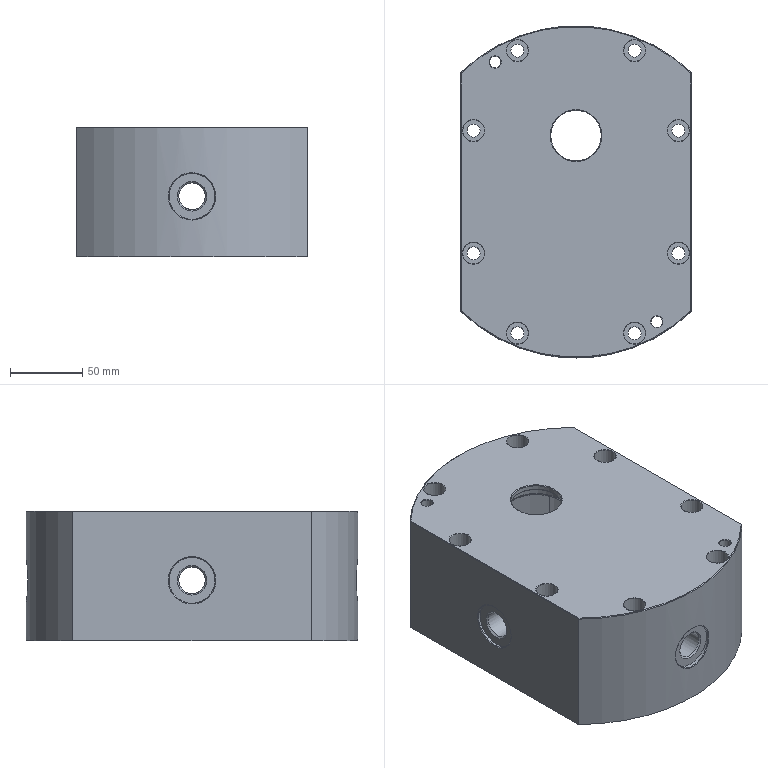NC program | NX | posted with a generic post | part box 160 x 230 x 90 mm
Lines 992 to 2004 of 9223:
(FLOOR_WALL_1 , TOOL : D25R0.5)
N1946 T05 M6
N1948 G54
N1950 G17 G0 G90 X38.751 Y-10.4 B0. C0. S2000 M3
N1952 G43 Z30. H5
N1954 Z1.5
N1956 G94 G1 X44.193 Z1.358 F1000.
N1958 X44.411 Y-9.472 Z1.333
N1960 X44.847 Y-7.127 Z1.27
N1962 X45.16 Y-4.762 Z1.208
N1964 X45.347 Y-2.385 Z1.145
N1966 X45.41 Y0. Z1.083
N1968 X45.347 Y2.385 Z1.02
N1970 X45.16 Y4.762 Z0.958
N1972 X44.847 Y7.127 Z0.895
N1974 X44.411 Y9.472 Z0.833
N1976 X44.193 Y10.4 Z0.808
N1978 X0. Z-0.349
N1980 X-44.193 F2200.
N1982 G3 X-44.193 Y-10.4 R45.4
N1984 G1 X44.193
N1986 G3 X44.193 Y10.4 R45.4
N1988 G1 X0.
N1990 Y27.9
N1992 X-56.374
N1994 G3 X-56.374 Y-27.9 R62.9
N1996 G1 X56.374
N1998 G3 X56.374 Y27.9 R62.9
N2000 G1 X0.
N2002 Y45.4
N2004 X-65.077
N2006 G3 X-67.079 Y44.323 R2.4
N2008 X-67.079 Y-44.323 R80.4
N2010 X-65.077 Y-45.4 R2.4
N2012 G1 X65.077
N2014 G3 X67.079 Y-44.323 R2.4
N2016 X67.079 Y44.323 R80.4
N2018 X65.077 Y45.4 R2.4
N2020 G1 X0.
N2022 Z1.151
N2024 G0 X38.751 Y-10.4
N2026 G1 X44.193 Z1.008 F1000.
N2028 X44.411 Y-9.472 Z0.983
N2030 X44.847 Y-7.127 Z0.921
N2032 X45.16 Y-4.762 Z0.858
N2034 X45.347 Y-2.385 Z0.796
N2036 X45.41 Y0. Z0.733
N2038 X45.347 Y2.385 Z0.671
N2040 X45.16 Y4.762 Z0.608
N2042 X44.847 Y7.127 Z0.546
N2044 X44.411 Y9.472 Z0.484
N2046 X44.193 Y10.4 Z0.459
N2048 X0. Z-0.699
N2050 X-44.193 F2200.
N2052 G3 X-44.193 Y-10.4 R45.4
N2054 G1 X44.193
N2056 G3 X44.193 Y10.4 R45.4
N2058 G1 X0.
N2060 Y27.9
N2062 X-56.374
N2064 G3 X-56.374 Y-27.9 R62.9
N2066 G1 X56.374
N2068 G3 X56.374 Y27.9 R62.9
N2070 G1 X0.
N2072 Y45.4
N2074 X-65.077
N2076 G3 X-67.079 Y44.323 R2.4
N2078 X-67.079 Y-44.323 R80.4
N2080 X-65.077 Y-45.4 R2.4
N2082 G1 X65.077
N2084 G3 X67.079 Y-44.323 R2.4
N2086 X67.079 Y44.323 R80.4
N2088 X65.077 Y45.4 R2.4
N2090 G1 X0.
N2092 Z0.801
N2094 G0 X38.751 Y-10.4
N2096 G1 X44.193 Z0.659 F1000.
N2098 X44.411 Y-9.472 Z0.634
N2100 X44.847 Y-7.127 Z0.571
N2102 X45.16 Y-4.762 Z0.509
N2104 X45.347 Y-2.385 Z0.447
N2106 X45.41 Y0. Z0.384
N2108 X45.347 Y2.385 Z0.322
N2110 X45.16 Y4.762 Z0.259
N2112 X44.847 Y7.127 Z0.197
N2114 X44.411 Y9.472 Z0.134
N2116 X44.193 Y10.4 Z0.109
N2118 X0. Z-1.048
N2120 X-44.193 F2200.
N2122 G3 X-44.193 Y-10.4 R45.4
N2124 G1 X44.193
N2126 G3 X44.193 Y10.4 R45.4
N2128 G1 X0.
N2130 Y27.9
N2132 X-56.374
N2134 G3 X-56.374 Y-27.9 R62.9
N2136 G1 X56.374
N2138 G3 X56.374 Y27.9 R62.9
N2140 G1 X0.
N2142 Y45.4
N2144 X-65.077
N2146 G3 X-67.079 Y44.323 R2.4
N2148 X-67.079 Y-44.323 R80.4
N2150 X-65.077 Y-45.4 R2.4
N2152 G1 X65.077
N2154 G3 X67.079 Y-44.323 R2.4
N2156 X67.079 Y44.323 R80.4
N2158 X65.077 Y45.4 R2.4
N2160 G1 X0.
N2162 Z0.452
N2164 G0 X38.751 Y-10.4
N2166 G1 X44.193 Z0.31 F1000.
N2168 X44.411 Y-9.472 Z0.285
N2170 X44.847 Y-7.127 Z0.222
N2172 X45.16 Y-4.762 Z0.16
N2174 X45.347 Y-2.385 Z0.097
N2176 X45.41 Y0. Z0.035
N2178 X45.347 Y2.385 Z-0.028
N2180 X45.16 Y4.762 Z-0.09
N2182 X44.847 Y7.127 Z-0.153
N2184 X44.411 Y9.472 Z-0.215
N2186 X44.193 Y10.4 Z-0.24
N2188 X0. Z-1.397
N2190 X-44.193 F2200.
N2192 G3 X-44.193 Y-10.4 R45.4
N2194 G1 X44.193
N2196 G3 X44.193 Y10.4 R45.4
N2198 G1 X0.
N2200 Y27.9
N2202 X-56.374
N2204 G3 X-56.374 Y-27.9 R62.9
N2206 G1 X56.374
N2208 G3 X56.374 Y27.9 R62.9
N2210 G1 X0.
N2212 Y45.4
N2214 X-65.077
N2216 G3 X-67.079 Y44.323 R2.4
N2218 X-67.079 Y-44.323 R80.4
N2220 X-65.077 Y-45.4 R2.4
N2222 G1 X65.077
N2224 G3 X67.079 Y-44.323 R2.4
N2226 X67.079 Y44.323 R80.4
N2228 X65.077 Y45.4 R2.4
N2230 G1 X0.
N2232 Z0.103
N2234 G0 X38.751 Y-10.4
N2236 G1 X44.193 Z-0.04 F1000.
N2238 X44.411 Y-9.472 Z-0.065
N2240 X44.847 Y-7.127 Z-0.127
N2242 X45.16 Y-4.762 Z-0.19
N2244 X45.347 Y-2.385 Z-0.252
N2246 X45.41 Y0. Z-0.315
N2248 X45.347 Y2.385 Z-0.377
N2250 X45.16 Y4.762 Z-0.44
N2252 X44.847 Y7.127 Z-0.502
N2254 X44.411 Y9.472 Z-0.564
N2256 X44.193 Y10.4 Z-0.589
N2258 X0. Z-1.747
N2260 X-44.193 F2200.
N2262 G3 X-44.193 Y-10.4 R45.4
N2264 G1 X44.193
N2266 G3 X44.193 Y10.4 R45.4
N2268 G1 X0.
N2270 Y27.9
N2272 X-56.374
N2274 G3 X-56.374 Y-27.9 R62.9
N2276 G1 X56.374
N2278 G3 X56.374 Y27.9 R62.9
N2280 G1 X0.
N2282 Y45.4
N2284 X-65.077
N2286 G3 X-67.079 Y44.323 R2.4
N2288 X-67.079 Y-44.323 R80.4
N2290 X-65.077 Y-45.4 R2.4
N2292 G1 X65.077
N2294 G3 X67.079 Y-44.323 R2.4
N2296 X67.079 Y44.323 R80.4
N2298 X65.077 Y45.4 R2.4
N2300 G1 X0.
N2302 Z-0.247
N2304 G0 X38.751 Y-10.4
N2306 G1 X44.193 Z-0.389 F1000.
N2308 X44.411 Y-9.472 Z-0.414
N2310 X44.847 Y-7.127 Z-0.477
N2312 X45.16 Y-4.762 Z-0.539
N2314 X45.347 Y-2.385 Z-0.601
N2316 X45.41 Y0. Z-0.664
N2318 X45.347 Y2.385 Z-0.726
N2320 X45.16 Y4.762 Z-0.789
N2322 X44.847 Y7.127 Z-0.851
N2324 X44.411 Y9.472 Z-0.914
N2326 X44.193 Y10.4 Z-0.939
N2328 X0. Z-2.096
N2330 X-44.193 F2200.
N2332 G3 X-44.193 Y-10.4 R45.4
N2334 G1 X44.193
N2336 G3 X44.193 Y10.4 R45.4
N2338 G1 X0.
N2340 Y27.9
N2342 X-56.374
N2344 G3 X-56.374 Y-27.9 R62.9
N2346 G1 X56.374
N2348 G3 X56.374 Y27.9 R62.9
N2350 G1 X0.
N2352 Y45.4
N2354 X-65.077
N2356 G3 X-67.079 Y44.323 R2.4
N2358 X-67.079 Y-44.323 R80.4
N2360 X-65.077 Y-45.4 R2.4
N2362 G1 X65.077
N2364 G3 X67.079 Y-44.323 R2.4
N2366 X67.079 Y44.323 R80.4
N2368 X65.077 Y45.4 R2.4
N2370 G1 X0.
N2372 Z-0.596
N2374 G0 X38.751 Y-10.4
N2376 G1 X44.193 Z-0.738 F1000.
N2378 X44.411 Y-9.472 Z-0.763
N2380 X44.847 Y-7.127 Z-0.826
N2382 X45.16 Y-4.762 Z-0.888
N2384 X45.347 Y-2.385 Z-0.951
N2386 X45.41 Y0. Z-1.013
N2388 X45.347 Y2.385 Z-1.076
N2390 X45.16 Y4.762 Z-1.138
N2392 X44.847 Y7.127 Z-1.201
N2394 X44.411 Y9.472 Z-1.263
N2396 X44.193 Y10.4 Z-1.288
N2398 X0. Z-2.445
N2400 X-44.193 F2200.
N2402 G3 X-44.193 Y-10.4 R45.4
N2404 G1 X44.193
N2406 G3 X44.193 Y10.4 R45.4
N2408 G1 X0.
N2410 Y27.9
N2412 X-56.374
N2414 G3 X-56.374 Y-27.9 R62.9
N2416 G1 X56.374
N2418 G3 X56.374 Y27.9 R62.9
N2420 G1 X0.
N2422 Y45.4
N2424 X-65.077
N2426 G3 X-67.079 Y44.323 R2.4
N2428 X-67.079 Y-44.323 R80.4
N2430 X-65.077 Y-45.4 R2.4
N2432 G1 X65.077
N2434 G3 X67.079 Y-44.323 R2.4
N2436 X67.079 Y44.323 R80.4
N2438 X65.077 Y45.4 R2.4
N2440 G1 X0.
N2442 Z-0.945
N2444 G0 X38.751 Y-10.4
N2446 G1 X44.193 Z-1.088 F1000.
N2448 X44.411 Y-9.472 Z-1.113
N2450 X44.847 Y-7.127 Z-1.175
N2452 X45.16 Y-4.762 Z-1.238
N2454 X45.347 Y-2.385 Z-1.3
N2456 X45.41 Y0. Z-1.363
N2458 X45.347 Y2.385 Z-1.425
N2460 X45.16 Y4.762 Z-1.488
N2462 X44.847 Y7.127 Z-1.55
N2464 X44.411 Y9.472 Z-1.612
N2466 X44.193 Y10.4 Z-1.637
N2468 X0. Z-2.795
N2470 X-44.193 F2200.
N2472 G3 X-44.193 Y-10.4 R45.4
N2474 G1 X44.193
N2476 G3 X44.193 Y10.4 R45.4
N2478 G1 X0.
N2480 Y27.9
N2482 X-56.374
N2484 G3 X-56.374 Y-27.9 R62.9
N2486 G1 X56.374
N2488 G3 X56.374 Y27.9 R62.9
N2490 G1 X0.
N2492 Y45.4
N2494 X-65.077
N2496 G3 X-67.079 Y44.323 R2.4
N2498 X-67.079 Y-44.323 R80.4
N2500 X-65.077 Y-45.4 R2.4
N2502 G1 X65.077
N2504 G3 X67.079 Y-44.323 R2.4
N2506 X67.079 Y44.323 R80.4
N2508 X65.077 Y45.4 R2.4
N2510 G1 X0.
N2512 Z-1.295
N2514 G0 X38.751 Y-10.4
N2516 G1 X44.193 Z-1.437 F1000.
N2518 X44.411 Y-9.472 Z-1.462
N2520 X44.847 Y-7.127 Z-1.525
N2522 X45.16 Y-4.762 Z-1.587
N2524 X45.347 Y-2.385 Z-1.649
N2526 X45.41 Y0. Z-1.712
N2528 X45.347 Y2.385 Z-1.774
N2530 X45.16 Y4.762 Z-1.837
N2532 X44.847 Y7.127 Z-1.899
N2534 X44.411 Y9.472 Z-1.962
N2536 X44.193 Y10.4 Z-1.987
N2538 X0. Z-3.144
N2540 X-44.193 F2200.
N2542 G3 X-44.193 Y-10.4 R45.4
N2544 G1 X44.193
N2546 G3 X44.193 Y10.4 R45.4
N2548 G1 X0.
N2550 Y27.9
N2552 X-56.374
N2554 G3 X-56.374 Y-27.9 R62.9
N2556 G1 X56.374
N2558 G3 X56.374 Y27.9 R62.9
N2560 G1 X0.
N2562 Y45.4
N2564 X-65.077
N2566 G3 X-67.079 Y44.323 R2.4
N2568 X-67.079 Y-44.323 R80.4
N2570 X-65.077 Y-45.4 R2.4
N2572 G1 X65.077
N2574 G3 X67.079 Y-44.323 R2.4
N2576 X67.079 Y44.323 R80.4
N2578 X65.077 Y45.4 R2.4
N2580 G1 X0.
N2582 Z-1.644
N2584 G0 X38.751 Y-10.4
N2586 G1 X44.193 Z-1.786 F1000.
N2588 X44.411 Y-9.472 Z-1.811
N2590 X44.847 Y-7.127 Z-1.874
N2592 X45.16 Y-4.762 Z-1.936
N2594 X45.347 Y-2.385 Z-1.999
N2596 X45.41 Y0. Z-2.061
N2598 X45.347 Y2.385 Z-2.124
N2600 X45.16 Y4.762 Z-2.186
N2602 X44.847 Y7.127 Z-2.249
N2604 X44.411 Y9.472 Z-2.311
N2606 X44.193 Y10.4 Z-2.336
N2608 X0. Z-3.493
N2610 X-44.193 F2200.
N2612 G3 X-44.193 Y-10.4 R45.4
N2614 G1 X44.193
N2616 G3 X44.193 Y10.4 R45.4
N2618 G1 X0.
N2620 Y27.9
N2622 X-56.374
N2624 G3 X-56.374 Y-27.9 R62.9
N2626 G1 X56.374
N2628 G3 X56.374 Y27.9 R62.9
N2630 G1 X0.
N2632 Y45.4
N2634 X-65.077
N2636 G3 X-67.079 Y44.323 R2.4
N2638 X-67.079 Y-44.323 R80.4
N2640 X-65.077 Y-45.4 R2.4
N2642 G1 X65.077
N2644 G3 X67.079 Y-44.323 R2.4
N2646 X67.079 Y44.323 R80.4
N2648 X65.077 Y45.4 R2.4
N2650 G1 X0.
N2652 Z-1.993
N2654 G0 X38.751 Y-10.4
N2656 G1 X44.193 Z-2.136 F1000.
N2658 X44.411 Y-9.472 Z-2.161
N2660 X44.847 Y-7.127 Z-2.223
N2662 X45.16 Y-4.762 Z-2.286
N2664 X45.347 Y-2.385 Z-2.348
N2666 X45.41 Y0. Z-2.411
N2668 X45.347 Y2.385 Z-2.473
N2670 X45.16 Y4.762 Z-2.535
N2672 X44.847 Y7.127 Z-2.598
N2674 X44.411 Y9.472 Z-2.66
N2676 X44.193 Y10.4 Z-2.685
N2678 X0. Z-3.843
N2680 X-44.193 F2200.
N2682 G3 X-44.193 Y-10.4 R45.4
N2684 G1 X44.193
N2686 G3 X44.193 Y10.4 R45.4
N2688 G1 X0.
N2690 Y27.9
N2692 X-56.374
N2694 G3 X-56.374 Y-27.9 R62.9
N2696 G1 X56.374
N2698 G3 X56.374 Y27.9 R62.9
N2700 G1 X0.
N2702 Y45.4
N2704 X-65.077
N2706 G3 X-67.079 Y44.323 R2.4
N2708 X-67.079 Y-44.323 R80.4
N2710 X-65.077 Y-45.4 R2.4
N2712 G1 X65.077
N2714 G3 X67.079 Y-44.323 R2.4
N2716 X67.079 Y44.323 R80.4
N2718 X65.077 Y45.4 R2.4
N2720 G1 X0.
N2722 Z-2.343
N2724 G0 X38.751 Y-10.4
N2726 G1 X44.193 Z-2.485 F1000.
N2728 X44.411 Y-9.472 Z-2.51
N2730 X44.847 Y-7.127 Z-2.573
N2732 X45.16 Y-4.762 Z-2.635
N2734 X45.347 Y-2.385 Z-2.697
N2736 X45.41 Y0. Z-2.76
N2738 X45.347 Y2.385 Z-2.822
N2740 X45.16 Y4.762 Z-2.885
N2742 X44.847 Y7.127 Z-2.947
N2744 X44.411 Y9.472 Z-3.01
N2746 X44.193 Y10.4 Z-3.035
N2748 X0. Z-4.192
N2750 X-44.193 F2200.
N2752 G3 X-44.193 Y-10.4 R45.4
N2754 G1 X44.193
N2756 G3 X44.193 Y10.4 R45.4
N2758 G1 X0.
N2760 Y27.9
N2762 X-56.374
N2764 G3 X-56.374 Y-27.9 R62.9
N2766 G1 X56.374
N2768 G3 X56.374 Y27.9 R62.9
N2770 G1 X0.
N2772 Y45.4
N2774 X-65.077
N2776 G3 X-67.079 Y44.323 R2.4
N2778 X-67.079 Y-44.323 R80.4
N2780 X-65.077 Y-45.4 R2.4
N2782 G1 X65.077
N2784 G3 X67.079 Y-44.323 R2.4
N2786 X67.079 Y44.323 R80.4
N2788 X65.077 Y45.4 R2.4
N2790 G1 X0.
N2792 Z-2.692
N2794 G0 X38.751 Y-10.4
N2796 G1 X44.193 Z-2.834 F1000.
N2798 X44.411 Y-9.472 Z-2.859
N2800 X44.847 Y-7.127 Z-2.922
N2802 X45.16 Y-4.762 Z-2.984
N2804 X45.347 Y-2.385 Z-3.047
N2806 X45.41 Y0. Z-3.109
N2808 X45.347 Y2.385 Z-3.172
N2810 X45.16 Y4.762 Z-3.234
N2812 X44.847 Y7.127 Z-3.297
N2814 X44.411 Y9.472 Z-3.359
N2816 X44.193 Y10.4 Z-3.384
N2818 X0. Z-4.541
N2820 X-44.193 F2200.
N2822 G3 X-44.193 Y-10.4 R45.4
N2824 G1 X44.193
N2826 G3 X44.193 Y10.4 R45.4
N2828 G1 X0.
N2830 Y27.9
N2832 X-56.374
N2834 G3 X-56.374 Y-27.9 R62.9
N2836 G1 X56.374
N2838 G3 X56.374 Y27.9 R62.9
N2840 G1 X0.
N2842 Y45.4
N2844 X-65.077
N2846 G3 X-67.079 Y44.323 R2.4
N2848 X-67.079 Y-44.323 R80.4
N2850 X-65.077 Y-45.4 R2.4
N2852 G1 X65.077
N2854 G3 X67.079 Y-44.323 R2.4
N2856 X67.079 Y44.323 R80.4
N2858 X65.077 Y45.4 R2.4
N2860 G1 X0.
N2862 Z-3.041
N2864 G0 X38.751 Y-10.4
N2866 G1 X44.193 Z-3.184 F1000.
N2868 X44.411 Y-9.472 Z-3.209
N2870 X44.847 Y-7.127 Z-3.271
N2872 X45.16 Y-4.762 Z-3.334
N2874 X45.347 Y-2.385 Z-3.396
N2876 X45.41 Y0. Z-3.459
N2878 X45.347 Y2.385 Z-3.521
N2880 X45.16 Y4.762 Z-3.583
N2882 X44.847 Y7.127 Z-3.646
N2884 X44.411 Y9.472 Z-3.708
N2886 X44.193 Y10.4 Z-3.733
N2888 X0. Z-4.891
N2890 X-44.193 F2200.
N2892 G3 X-44.193 Y-10.4 R45.4
N2894 G1 X44.193
N2896 G3 X44.193 Y10.4 R45.4
N2898 G1 X0.
N2900 Y27.9
N2902 X-56.374
N2904 G3 X-56.374 Y-27.9 R62.9
N2906 G1 X56.374
N2908 G3 X56.374 Y27.9 R62.9
N2910 G1 X0.
N2912 Y45.4
N2914 X-65.077
N2916 G3 X-67.079 Y44.323 R2.4
N2918 X-67.079 Y-44.323 R80.4
N2920 X-65.077 Y-45.4 R2.4
N2922 G1 X65.077
N2924 G3 X67.079 Y-44.323 R2.4
N2926 X67.079 Y44.323 R80.4
N2928 X65.077 Y45.4 R2.4
N2930 G1 X0.
N2932 Z-3.391
N2934 G0 X38.751 Y-10.4
N2936 G1 X44.193 Z-3.533 F1000.
N2938 X44.411 Y-9.472 Z-3.558
N2940 X44.847 Y-7.127 Z-3.62
N2942 X45.16 Y-4.762 Z-3.683
N2944 X45.347 Y-2.385 Z-3.745
N2946 X45.41 Y0. Z-3.808
N2948 X45.347 Y2.385 Z-3.87
N2950 X45.16 Y4.762 Z-3.933
N2952 X44.847 Y7.127 Z-3.995
N2954 X44.411 Y9.472 Z-4.058
N2956 X44.193 Y10.4 Z-4.083
N2958 X0. Z-5.24
N2960 X-44.193 F2200.
N2962 G3 X-44.193 Y-10.4 R45.4
N2964 G1 X44.193
N2966 G3 X44.193 Y10.4 R45.4
N2968 G1 X0.
N2970 Y27.9
N2972 X-56.374
N2974 G3 X-56.374 Y-27.9 R62.9
N2976 G1 X56.374
N2978 G3 X56.374 Y27.9 R62.9
N2980 G1 X0.
N2982 Y45.4
N2984 X-65.077
N2986 G3 X-67.079 Y44.323 R2.4
N2988 X-67.079 Y-44.323 R80.4
N2990 X-65.077 Y-45.4 R2.4
N2992 G1 X65.077
N2994 G3 X67.079 Y-44.323 R2.4
N2996 X67.079 Y44.323 R80.4
N2998 X65.077 Y45.4 R2.4
N3000 G1 X0.
N3002 Z-3.74
N3004 G0 X38.751 Y-10.4
N3006 G1 X44.193 Z-3.882 F1000.
N3008 X44.411 Y-9.472 Z-3.907
N3010 X44.847 Y-7.127 Z-3.97
N3012 X45.16 Y-4.762 Z-4.032
N3014 X45.347 Y-2.385 Z-4.095
N3016 X45.41 Y0. Z-4.157
N3018 X45.347 Y2.385 Z-4.22
N3020 X45.16 Y4.762 Z-4.282
N3022 X44.847 Y7.127 Z-4.345
N3024 X44.411 Y9.472 Z-4.407
N3026 X44.193 Y10.4 Z-4.432
N3028 X0. Z-5.589
N3030 X-44.193 F2200.
N3032 G3 X-44.193 Y-10.4 R45.4
N3034 G1 X44.193
N3036 G3 X44.193 Y10.4 R45.4
N3038 G1 X0.
N3040 Y27.9
N3042 X-56.374
N3044 G3 X-56.374 Y-27.9 R62.9
N3046 G1 X56.374
N3048 G3 X56.374 Y27.9 R62.9
N3050 G1 X0.
N3052 Y45.4
N3054 X-65.077
N3056 G3 X-67.079 Y44.323 R2.4
N3058 X-67.079 Y-44.323 R80.4
N3060 X-65.077 Y-45.4 R2.4
N3062 G1 X65.077
N3064 G3 X67.079 Y-44.323 R2.4
N3066 X67.079 Y44.323 R80.4
N3068 X65.077 Y45.4 R2.4
N3070 G1 X0.
N3072 Z-4.089
N3074 G0 X38.751 Y-10.4
N3076 G1 X44.193 Z-4.232 F1000.
N3078 X44.411 Y-9.472 Z-4.257
N3080 X44.847 Y-7.127 Z-4.319
N3082 X45.16 Y-4.762 Z-4.382
N3084 X45.347 Y-2.385 Z-4.444
N3086 X45.41 Y0. Z-4.507
N3088 X45.347 Y2.385 Z-4.569
N3090 X45.16 Y4.762 Z-4.631
N3092 X44.847 Y7.127 Z-4.694
N3094 X44.411 Y9.472 Z-4.756
N3096 X44.193 Y10.4 Z-4.781
N3098 X0. Z-5.939
N3100 X-44.193 F2200.
N3102 G3 X-44.193 Y-10.4 R45.4
N3104 G1 X44.193
N3106 G3 X44.193 Y10.4 R45.4
N3108 G1 X0.
N3110 Y27.9
N3112 X-56.374
N3114 G3 X-56.374 Y-27.9 R62.9
N3116 G1 X56.374
N3118 G3 X56.374 Y27.9 R62.9
N3120 G1 X0.
N3122 Y45.4
N3124 X-65.077
N3126 G3 X-67.079 Y44.323 R2.4
N3128 X-67.079 Y-44.323 R80.4
N3130 X-65.077 Y-45.4 R2.4
N3132 G1 X65.077
N3134 G3 X67.079 Y-44.323 R2.4
N3136 X67.079 Y44.323 R80.4
N3138 X65.077 Y45.4 R2.4
N3140 G1 X0.
N3142 Z-4.439
N3144 G0 X38.751 Y-10.4
N3146 G1 X44.193 Z-4.581 F1000.
N3148 X44.411 Y-9.472 Z-4.606
N3150 X44.847 Y-7.127 Z-4.668
N3152 X45.16 Y-4.762 Z-4.731
N3154 X45.347 Y-2.385 Z-4.793
N3156 X45.41 Y0. Z-4.856
N3158 X45.347 Y2.385 Z-4.918
N3160 X45.16 Y4.762 Z-4.981
N3162 X44.847 Y7.127 Z-5.043
N3164 X44.411 Y9.472 Z-5.106
N3166 X44.193 Y10.4 Z-5.131
N3168 X0. Z-6.288
N3170 X-44.193 F2200.
N3172 G3 X-44.193 Y-10.4 R45.4
N3174 G1 X44.193
N3176 G3 X44.193 Y10.4 R45.4
N3178 G1 X0.
N3180 Y27.9
N3182 X-56.374
N3184 G3 X-56.374 Y-27.9 R62.9
N3186 G1 X56.374
N3188 G3 X56.374 Y27.9 R62.9
N3190 G1 X0.
N3192 Y45.4
N3194 X-65.077
N3196 G3 X-67.079 Y44.323 R2.4
N3198 X-67.079 Y-44.323 R80.4
N3200 X-65.077 Y-45.4 R2.4
N3202 G1 X65.077
N3204 G3 X67.079 Y-44.323 R2.4
N3206 X67.079 Y44.323 R80.4
N3208 X65.077 Y45.4 R2.4
N3210 G1 X0.
N3212 Z-4.788
N3214 G0 X38.751 Y-10.4
N3216 G1 X44.193 Z-4.93 F1000.
N3218 X44.411 Y-9.472 Z-4.955
N3220 X44.847 Y-7.127 Z-5.018
N3222 X45.16 Y-4.762 Z-5.08
N3224 X45.347 Y-2.385 Z-5.143
N3226 X45.41 Y0. Z-5.205
N3228 X45.347 Y2.385 Z-5.268
N3230 X45.16 Y4.762 Z-5.33
N3232 X44.847 Y7.127 Z-5.393
N3234 X44.411 Y9.472 Z-5.455
N3236 X44.193 Y10.4 Z-5.48
N3238 X0. Z-6.637
N3240 X-44.193 F2200.
N3242 G3 X-44.193 Y-10.4 R45.4
N3244 G1 X44.193
N3246 G3 X44.193 Y10.4 R45.4
N3248 G1 X0.
N3250 Y27.9
N3252 X-56.374
N3254 G3 X-56.374 Y-27.9 R62.9
N3256 G1 X56.374
N3258 G3 X56.374 Y27.9 R62.9
N3260 G1 X0.
N3262 Y45.4
N3264 X-65.077
N3266 G3 X-67.079 Y44.323 R2.4
N3268 X-67.079 Y-44.323 R80.4
N3270 X-65.077 Y-45.4 R2.4
N3272 G1 X65.077
N3274 G3 X67.079 Y-44.323 R2.4
N3276 X67.079 Y44.323 R80.4
N3278 X65.077 Y45.4 R2.4
N3280 G1 X0.
N3282 Z-5.137
N3284 G0 X38.751 Y-10.4
N3286 G1 X44.193 Z-5.28 F1000.
N3288 X44.411 Y-9.472 Z-5.305
N3290 X44.847 Y-7.127 Z-5.367
N3292 X45.16 Y-4.762 Z-5.43
N3294 X45.347 Y-2.385 Z-5.492
N3296 X45.41 Y0. Z-5.555
N3298 X45.347 Y2.385 Z-5.617
N3300 X45.16 Y4.762 Z-5.679
N3302 X44.847 Y7.127 Z-5.742
N3304 X44.411 Y9.472 Z-5.804
N3306 X44.193 Y10.4 Z-5.829
N3308 X0. Z-6.987
N3310 X-44.193 F2200.
N3312 G3 X-44.193 Y-10.4 R45.4
N3314 G1 X44.193
N3316 G3 X44.193 Y10.4 R45.4
N3318 G1 X0.
N3320 Y27.9
N3322 X-56.374
N3324 G3 X-56.374 Y-27.9 R62.9
N3326 G1 X56.374
N3328 G3 X56.374 Y27.9 R62.9
N3330 G1 X0.
N3332 Y45.4
N3334 X-65.077
N3336 G3 X-67.079 Y44.323 R2.4
N3338 X-67.079 Y-44.323 R80.4
N3340 X-65.077 Y-45.4 R2.4
N3342 G1 X65.077
N3344 G3 X67.079 Y-44.323 R2.4
N3346 X67.079 Y44.323 R80.4
N3348 X65.077 Y45.4 R2.4
N3350 G1 X0.
N3352 Z-5.487
N3354 G0 X38.751 Y-10.4
N3356 G1 X44.193 Z-5.629 F1000.
N3358 X44.411 Y-9.472 Z-5.654
N3360 X44.847 Y-7.127 Z-5.716
N3362 X45.16 Y-4.762 Z-5.779
N3364 X45.347 Y-2.385 Z-5.841
N3366 X45.41 Y0. Z-5.904
N3368 X45.347 Y2.385 Z-5.966
N3370 X45.16 Y4.762 Z-6.029
N3372 X44.847 Y7.127 Z-6.091
N3374 X44.411 Y9.472 Z-6.154
N3376 X44.193 Y10.4 Z-6.179
N3378 X0. Z-7.336
N3380 X-44.193 F2200.
N3382 G3 X-44.193 Y-10.4 R45.4
N3384 G1 X44.193
N3386 G3 X44.193 Y10.4 R45.4
N3388 G1 X0.
N3390 Y27.9
N3392 X-56.374
N3394 G3 X-56.374 Y-27.9 R62.9
N3396 G1 X56.374
N3398 G3 X56.374 Y27.9 R62.9
N3400 G1 X0.
N3402 Y45.4
N3404 X-65.077
N3406 G3 X-67.079 Y44.323 R2.4
N3408 X-67.079 Y-44.323 R80.4
N3410 X-65.077 Y-45.4 R2.4
N3412 G1 X65.077
N3414 G3 X67.079 Y-44.323 R2.4
N3416 X67.079 Y44.323 R80.4
N3418 X65.077 Y45.4 R2.4
N3420 G1 X0.
N3422 Z-5.836
N3424 G0 X38.751 Y-10.4
N3426 G1 X44.193 Z-5.978 F1000.
N3428 X44.411 Y-9.472 Z-6.003
N3430 X44.847 Y-7.127 Z-6.066
N3432 X45.16 Y-4.762 Z-6.128
N3434 X45.347 Y-2.385 Z-6.191
N3436 X45.41 Y0. Z-6.253
N3438 X45.347 Y2.385 Z-6.316
N3440 X45.16 Y4.762 Z-6.378
N3442 X44.847 Y7.127 Z-6.441
N3444 X44.411 Y9.472 Z-6.503
N3446 X44.193 Y10.4 Z-6.528
N3448 X0. Z-7.685
N3450 X-44.193 F2200.
N3452 G3 X-44.193 Y-10.4 R45.4
N3454 G1 X44.193
N3456 G3 X44.193 Y10.4 R45.4
N3458 G1 X0.
N3460 Y27.9
N3462 X-56.374
N3464 G3 X-56.374 Y-27.9 R62.9
N3466 G1 X56.374
N3468 G3 X56.374 Y27.9 R62.9
N3470 G1 X0.
N3472 Y45.4
N3474 X-65.077
N3476 G3 X-67.079 Y44.323 R2.4
N3478 X-67.079 Y-44.323 R80.4
N3480 X-65.077 Y-45.4 R2.4
N3482 G1 X65.077
N3484 G3 X67.079 Y-44.323 R2.4
N3486 X67.079 Y44.323 R80.4
N3488 X65.077 Y45.4 R2.4
N3490 G1 X0.
N3492 Z-6.185
N3494 G0 X38.751 Y-10.4
N3496 G1 X44.193 Z-6.328 F1000.
N3498 X44.411 Y-9.472 Z-6.353
N3500 X44.847 Y-7.127 Z-6.415
N3502 X45.16 Y-4.762 Z-6.478
N3504 X45.347 Y-2.385 Z-6.54
N3506 X45.41 Y0. Z-6.602
N3508 X45.347 Y2.385 Z-6.665
N3510 X45.16 Y4.762 Z-6.727
N3512 X44.847 Y7.127 Z-6.79
N3514 X44.411 Y9.472 Z-6.852
N3516 X44.193 Y10.4 Z-6.877
N3518 X0. Z-8.035
N3520 X-44.193 F2200.
N3522 G3 X-44.193 Y-10.4 R45.4
N3524 G1 X44.193
N3526 G3 X44.193 Y10.4 R45.4
N3528 G1 X0.
N3530 Y27.9
N3532 X-56.374
N3534 G3 X-56.374 Y-27.9 R62.9
N3536 G1 X56.374
N3538 G3 X56.374 Y27.9 R62.9
N3540 G1 X0.
N3542 Y45.4
N3544 X-65.077
N3546 G3 X-67.079 Y44.323 R2.4
N3548 X-67.079 Y-44.323 R80.4
N3550 X-65.077 Y-45.4 R2.4
N3552 G1 X65.077
N3554 G3 X67.079 Y-44.323 R2.4
N3556 X67.079 Y44.323 R80.4
N3558 X65.077 Y45.4 R2.4
N3560 G1 X0.
N3562 Z-6.535
N3564 G0 X38.751 Y-10.4
N3566 G1 X44.193 Z-6.677 F1000.
N3568 X44.411 Y-9.472 Z-6.702
N3570 X44.847 Y-7.127 Z-6.764
N3572 X45.16 Y-4.762 Z-6.827
N3574 X45.347 Y-2.385 Z-6.889
N3576 X45.41 Y0. Z-6.952
N3578 X45.347 Y2.385 Z-7.014
N3580 X45.16 Y4.762 Z-7.077
N3582 X44.847 Y7.127 Z-7.139
N3584 X44.411 Y9.472 Z-7.202
N3586 X44.193 Y10.4 Z-7.227
N3588 X0. Z-8.384
N3590 X-44.193 F2200.
N3592 G3 X-44.193 Y-10.4 R45.4
N3594 G1 X44.193
N3596 G3 X44.193 Y10.4 R45.4
N3598 G1 X0.
N3600 Y27.9
N3602 X-56.374
N3604 G3 X-56.374 Y-27.9 R62.9
N3606 G1 X56.374
N3608 G3 X56.374 Y27.9 R62.9
N3610 G1 X0.
N3612 Y45.4
N3614 X-65.077
N3616 G3 X-67.079 Y44.323 R2.4
N3618 X-67.079 Y-44.323 R80.4
N3620 X-65.077 Y-45.4 R2.4
N3622 G1 X65.077
N3624 G3 X67.079 Y-44.323 R2.4
N3626 X67.079 Y44.323 R80.4
N3628 X65.077 Y45.4 R2.4
N3630 G1 X0.
N3632 Z-6.884
N3634 G0 X38.751 Y-10.4
N3636 G1 X44.193 Z-7.026 F1000.
N3638 X44.411 Y-9.472 Z-7.051
N3640 X44.847 Y-7.127 Z-7.114
N3642 X45.16 Y-4.762 Z-7.176
N3644 X45.347 Y-2.385 Z-7.239
N3646 X45.41 Y0. Z-7.301
N3648 X45.347 Y2.385 Z-7.364
N3650 X45.16 Y4.762 Z-7.426
N3652 X44.847 Y7.127 Z-7.489
N3654 X44.411 Y9.472 Z-7.551
N3656 X44.193 Y10.4 Z-7.576
N3658 X0. Z-8.733
N3660 X-44.193 F2200.
N3662 G3 X-44.193 Y-10.4 R45.4
N3664 G1 X44.193
N3666 G3 X44.193 Y10.4 R45.4
N3668 G1 X0.
N3670 Y27.9
N3672 X-56.374
N3674 G3 X-56.374 Y-27.9 R62.9
N3676 G1 X56.374
N3678 G3 X56.374 Y27.9 R62.9
N3680 G1 X0.
N3682 Y45.4
N3684 X-65.077
N3686 G3 X-67.079 Y44.323 R2.4
N3688 X-67.079 Y-44.323 R80.4
N3690 X-65.077 Y-45.4 R2.4
N3692 G1 X65.077
N3694 G3 X67.079 Y-44.323 R2.4
N3696 X67.079 Y44.323 R80.4
N3698 X65.077 Y45.4 R2.4
N3700 G1 X0.
N3702 Z-7.233
N3704 G0 X38.751 Y-10.4
N3706 G1 X44.193 Z-7.376 F1000.
N3708 X44.411 Y-9.472 Z-7.401
N3710 X44.847 Y-7.127 Z-7.463
N3712 X45.16 Y-4.762 Z-7.526
N3714 X45.347 Y-2.385 Z-7.588
N3716 X45.41 Y0. Z-7.65
N3718 X45.347 Y2.385 Z-7.713
N3720 X45.16 Y4.762 Z-7.775
N3722 X44.847 Y7.127 Z-7.838
N3724 X44.411 Y9.472 Z-7.9
N3726 X44.193 Y10.4 Z-7.925
N3728 X0. Z-9.083
N3730 X-44.193 F2200.
N3732 G3 X-44.193 Y-10.4 R45.4
N3734 G1 X44.193
N3736 G3 X44.193 Y10.4 R45.4
N3738 G1 X0.
N3740 Y27.9
N3742 X-56.374
N3744 G3 X-56.374 Y-27.9 R62.9
N3746 G1 X56.374
N3748 G3 X56.374 Y27.9 R62.9
N3750 G1 X0.
N3752 Y45.4
N3754 X-65.077
N3756 G3 X-67.079 Y44.323 R2.4
N3758 X-67.079 Y-44.323 R80.4
N3760 X-65.077 Y-45.4 R2.4
N3762 G1 X65.077
N3764 G3 X67.079 Y-44.323 R2.4
N3766 X67.079 Y44.323 R80.4
N3768 X65.077 Y45.4 R2.4
N3770 G1 X0.
N3772 Z-7.583
N3774 G0 X38.751 Y-10.4
N3776 G1 X44.193 Z-7.725 F1000.
N3778 X44.411 Y-9.472 Z-7.75
N3780 X44.847 Y-7.127 Z-7.812
N3782 X45.16 Y-4.762 Z-7.875
N3784 X45.347 Y-2.385 Z-7.937
N3786 X45.41 Y0. Z-8.
N3788 X45.347 Y2.385 Z-8.062
N3790 X45.16 Y4.762 Z-8.125
N3792 X44.847 Y7.127 Z-8.187
N3794 X44.411 Y9.472 Z-8.25
N3796 X44.193 Y10.4 Z-8.275
N3798 X0. Z-9.432
N3800 X-44.193 F2200.
N3802 G3 X-44.193 Y-10.4 R45.4
N3804 G1 X44.193
N3806 G3 X44.193 Y10.4 R45.4
N3808 G1 X0.
N3810 Y27.9
N3812 X-56.374
N3814 G3 X-56.374 Y-27.9 R62.9
N3816 G1 X56.374
N3818 G3 X56.374 Y27.9 R62.9
N3820 G1 X0.
N3822 Y45.4
N3824 X-65.077
N3826 G3 X-67.079 Y44.323 R2.4
N3828 X-67.079 Y-44.323 R80.4
N3830 X-65.077 Y-45.4 R2.4
N3832 G1 X65.077
N3834 G3 X67.079 Y-44.323 R2.4
N3836 X67.079 Y44.323 R80.4
N3838 X65.077 Y45.4 R2.4
N3840 G1 X0.
N3842 Z-7.932
N3844 G0 X38.751 Y-10.4
N3846 G1 X44.193 Z-8.074 F1000.
N3848 X44.411 Y-9.472 Z-8.099
N3850 X44.847 Y-7.127 Z-8.162
N3852 X45.16 Y-4.762 Z-8.224
N3854 X45.347 Y-2.385 Z-8.287
N3856 X45.41 Y0. Z-8.349
N3858 X45.347 Y2.385 Z-8.412
N3860 X45.16 Y4.762 Z-8.474
N3862 X44.847 Y7.127 Z-8.537
N3864 X44.411 Y9.472 Z-8.599
N3866 X44.193 Y10.4 Z-8.624
N3868 X0. Z-9.781
N3870 X-44.193 F2200.
N3872 G3 X-44.193 Y-10.4 R45.4
N3874 G1 X44.193
N3876 G3 X44.193 Y10.4 R45.4
N3878 G1 X0.
N3880 Y27.9
N3882 X-56.374
N3884 G3 X-56.374 Y-27.9 R62.9
N3886 G1 X56.374
N3888 G3 X56.374 Y27.9 R62.9
N3890 G1 X0.
N3892 Y45.4
N3894 X-65.077
N3896 G3 X-67.079 Y44.323 R2.4
N3898 X-67.079 Y-44.323 R80.4
N3900 X-65.077 Y-45.4 R2.4
N3902 G1 X65.077
N3904 G3 X67.079 Y-44.323 R2.4
N3906 X67.079 Y44.323 R80.4
N3908 X65.077 Y45.4 R2.4
N3910 G1 X0.
N3912 Z-8.281
N3914 G0 X38.751 Y-10.4
N3916 G1 X44.193 Z-8.424 F1000.
N3918 X44.411 Y-9.472 Z-8.449
N3920 X44.847 Y-7.127 Z-8.511
N3922 X45.16 Y-4.762 Z-8.574
N3924 X45.347 Y-2.385 Z-8.636
N3926 X45.41 Y0. Z-8.698
N3928 X45.347 Y2.385 Z-8.761
N3930 X45.16 Y4.762 Z-8.823
N3932 X44.847 Y7.127 Z-8.886
N3934 X44.411 Y9.472 Z-8.948
N3936 X44.193 Y10.4 Z-8.973
N3938 X0. Z-10.13
N3940 X-44.193 F2200.
N3942 G3 X-44.193 Y-10.4 R45.4
N3944 G1 X44.193
N3946 G3 X44.193 Y10.4 R45.4
N3948 G1 X0.
N3950 Y27.9
N3952 X-56.374
N3954 G3 X-56.374 Y-27.9 R62.9
N3956 G1 X56.374
N3958 G3 X56.374 Y27.9 R62.9
N3960 G1 X0.
N3962 Y45.4
N3964 X-65.077